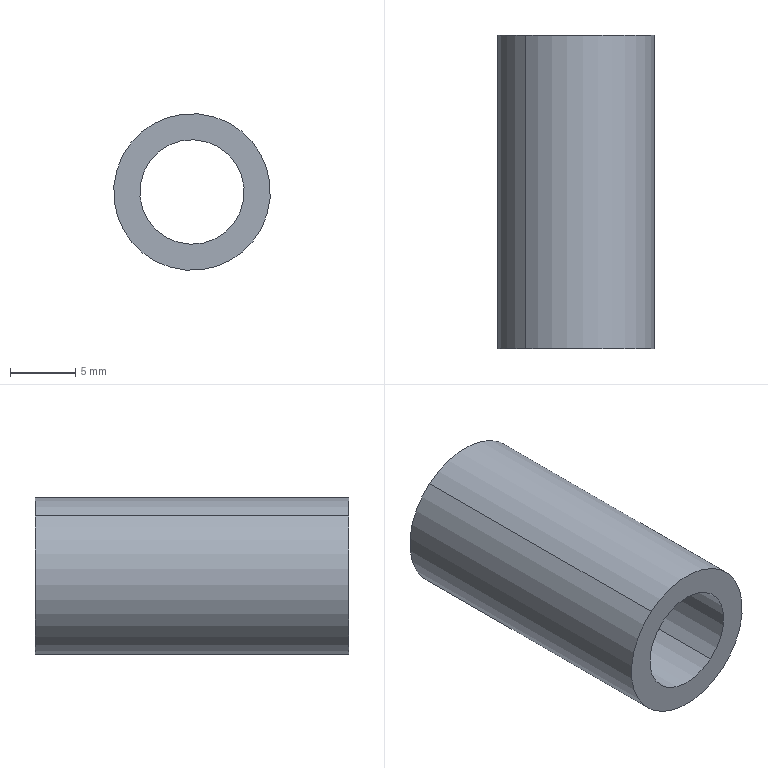Part | SolidWorks | features BaseBody 1 | 1 solid | 6 faces | box 12 x 24 x 12 mm | volume 1508 mm3 | cylinder 4 | plane 2 | commonest cylinder face diameters 8 x2 12 x2
STEP:
#1=CARTESIAN_POINT('',(374.241,-16.,154.364));
#2=VERTEX_POINT('',#1);
#3=CARTESIAN_POINT('',(379.383,-16.,148.236));
#4=VERTEX_POINT('',#3);
#5=CARTESIAN_POINT('',(376.812,-16.,151.3));
#6=DIRECTION('',(0.,1.,0.));
#7=DIRECTION('',(-0.6428,0.,0.766));
#8=AXIS2_PLACEMENT_3D('',#5,#6,#7);
#9=CIRCLE('',#8,4.);
#10=EDGE_CURVE('',#2,#4,#9,.T.);
#11=ORIENTED_EDGE('',*,*,#10,.F.);
#12=CARTESIAN_POINT('',(374.241,8.,154.364));
#13=VERTEX_POINT('',#12);
#14=CARTESIAN_POINT('',(374.241,-32.971,154.364));
#15=DIRECTION('',(0.,1.,0.));
#16=VECTOR('',#15,1000.);
#17=LINE('',#14,#16);
#18=EDGE_CURVE('',#2,#13,#17,.T.);
#19=ORIENTED_EDGE('',*,*,#18,.T.);
#20=CARTESIAN_POINT('',(379.383,8.,148.236));
#21=VERTEX_POINT('',#20);
#22=CARTESIAN_POINT('',(376.812,8.,151.3));
#23=DIRECTION('',(0.,-1.,0.));
#24=DIRECTION('',(0.6428,0.,-0.766));
#25=AXIS2_PLACEMENT_3D('',#22,#23,#24);
#26=CIRCLE('',#25,4.);
#27=EDGE_CURVE('',#21,#13,#26,.T.);
#28=ORIENTED_EDGE('',*,*,#27,.F.);
#29=CARTESIAN_POINT('',(379.383,-32.971,148.236));
#30=DIRECTION('',(0.,1.,0.));
#31=VECTOR('',#30,1000.);
#32=LINE('',#29,#31);
#33=EDGE_CURVE('',#4,#21,#32,.T.);
#34=ORIENTED_EDGE('',*,*,#33,.F.);
#35=EDGE_LOOP('',(#11,#19,#28,#34));
#36=FACE_OUTER_BOUND('',#35,.T.);
#37=CARTESIAN_POINT('',(376.812,-32.971,151.3));
#38=DIRECTION('',(0.,1.,0.));
#39=DIRECTION('',(0.6428,0.,-0.766));
#40=AXIS2_PLACEMENT_3D('',#37,#38,#39);
#41=CYLINDRICAL_SURFACE('',#40,4.);
#42=ADVANCED_FACE('',(#36),#41,.F.);
#43=CARTESIAN_POINT('',(372.956,-16.,155.896));
#44=VERTEX_POINT('',#43);
#45=CARTESIAN_POINT('',(380.669,-16.,146.704));
#46=VERTEX_POINT('',#45);
#47=CARTESIAN_POINT('',(376.812,-16.,151.3));
#48=DIRECTION('',(0.,-1.,0.));
#49=DIRECTION('',(-0.6428,0.,0.766));
#50=AXIS2_PLACEMENT_3D('',#47,#48,#49);
#51=CIRCLE('',#50,6.);
#52=EDGE_CURVE('',#44,#46,#51,.T.);
#53=ORIENTED_EDGE('',*,*,#52,.F.);
#54=CARTESIAN_POINT('',(372.956,8.,155.896));
#55=VERTEX_POINT('',#54);
#56=CARTESIAN_POINT('',(372.956,-32.971,155.896));
#57=DIRECTION('',(0.,1.,0.));
#58=VECTOR('',#57,1000.);
#59=LINE('',#56,#58);
#60=EDGE_CURVE('',#44,#55,#59,.T.);
#61=ORIENTED_EDGE('',*,*,#60,.T.);
#62=CARTESIAN_POINT('',(380.669,8.,146.704));
#63=VERTEX_POINT('',#62);
#64=CARTESIAN_POINT('',(376.812,8.,151.3));
#65=DIRECTION('',(0.,1.,0.));
#66=DIRECTION('',(-0.6428,0.,0.766));
#67=AXIS2_PLACEMENT_3D('',#64,#65,#66);
#68=CIRCLE('',#67,6.);
#69=EDGE_CURVE('',#63,#55,#68,.T.);
#70=ORIENTED_EDGE('',*,*,#69,.F.);
#71=CARTESIAN_POINT('',(380.669,-32.971,146.704));
#72=DIRECTION('',(0.,1.,0.));
#73=VECTOR('',#72,1000.);
#74=LINE('',#71,#73);
#75=EDGE_CURVE('',#46,#63,#74,.T.);
#76=ORIENTED_EDGE('',*,*,#75,.F.);
#77=EDGE_LOOP('',(#53,#61,#70,#76));
#78=FACE_OUTER_BOUND('',#77,.T.);
#79=CARTESIAN_POINT('',(376.812,-32.971,151.3));
#80=DIRECTION('',(0.,1.,0.));
#81=DIRECTION('',(0.6428,0.,-0.766));
#82=AXIS2_PLACEMENT_3D('',#79,#80,#81);
#83=CYLINDRICAL_SURFACE('',#82,6.);
#84=ADVANCED_FACE('',(#78),#83,.T.);
#85=ORIENTED_EDGE('',*,*,#27,.T.);
#86=CARTESIAN_POINT('',(376.812,8.,151.3));
#87=DIRECTION('',(0.,-1.,0.));
#88=DIRECTION('',(0.6428,0.,-0.766));
#89=AXIS2_PLACEMENT_3D('',#86,#87,#88);
#90=CIRCLE('',#89,4.);
#91=EDGE_CURVE('',#13,#21,#90,.T.);
#92=ORIENTED_EDGE('',*,*,#91,.T.);
#93=EDGE_LOOP('',(#85,#92));
#94=FACE_BOUND('',#93,.T.);
#95=ORIENTED_EDGE('',*,*,#69,.T.);
#96=CARTESIAN_POINT('',(376.812,8.,151.3));
#97=DIRECTION('',(0.,1.,0.));
#98=DIRECTION('',(-0.6428,0.,0.766));
#99=AXIS2_PLACEMENT_3D('',#96,#97,#98);
#100=CIRCLE('',#99,6.);
#101=EDGE_CURVE('',#55,#63,#100,.T.);
#102=ORIENTED_EDGE('',*,*,#101,.T.);
#103=EDGE_LOOP('',(#95,#102));
#104=FACE_OUTER_BOUND('',#103,.T.);
#105=CARTESIAN_POINT('',(376.812,8.,151.3));
#106=DIRECTION('',(0.,1.,0.));
#107=DIRECTION('',(1.,0.,0.));
#108=AXIS2_PLACEMENT_3D('',#105,#106,#107);
#109=PLANE('',#108);
#110=ADVANCED_FACE('',(#94,#104),#109,.T.);
#111=ORIENTED_EDGE('',*,*,#60,.F.);
#112=CARTESIAN_POINT('',(376.812,-16.,151.3));
#113=DIRECTION('',(0.,-1.,0.));
#114=DIRECTION('',(-0.6428,0.,0.766));
#115=AXIS2_PLACEMENT_3D('',#112,#113,#114);
#116=CIRCLE('',#115,6.);
#117=EDGE_CURVE('',#46,#44,#116,.T.);
#118=ORIENTED_EDGE('',*,*,#117,.F.);
#119=ORIENTED_EDGE('',*,*,#75,.T.);
#120=ORIENTED_EDGE('',*,*,#101,.F.);
#121=EDGE_LOOP('',(#111,#118,#119,#120));
#122=FACE_OUTER_BOUND('',#121,.T.);
#123=CARTESIAN_POINT('',(376.812,-32.971,151.3));
#124=DIRECTION('',(0.,1.,0.));
#125=DIRECTION('',(0.6428,0.,-0.766));
#126=AXIS2_PLACEMENT_3D('',#123,#124,#125);
#127=CYLINDRICAL_SURFACE('',#126,6.);
#128=ADVANCED_FACE('',(#122),#127,.T.);
#129=CARTESIAN_POINT('',(376.812,-16.,151.3));
#130=DIRECTION('',(0.,1.,0.));
#131=DIRECTION('',(-0.6428,0.,0.766));
#132=AXIS2_PLACEMENT_3D('',#129,#130,#131);
#133=CIRCLE('',#132,4.);
#134=EDGE_CURVE('',#4,#2,#133,.T.);
#135=ORIENTED_EDGE('',*,*,#134,.T.);
#136=ORIENTED_EDGE('',*,*,#10,.T.);
#137=EDGE_LOOP('',(#135,#136));
#138=FACE_BOUND('',#137,.T.);
#139=ORIENTED_EDGE('',*,*,#117,.T.);
#140=ORIENTED_EDGE('',*,*,#52,.T.);
#141=EDGE_LOOP('',(#139,#140));
#142=FACE_OUTER_BOUND('',#141,.T.);
#143=CARTESIAN_POINT('',(376.812,-16.,151.3));
#144=DIRECTION('',(0.,1.,0.));
#145=DIRECTION('',(1.,0.,0.));
#146=AXIS2_PLACEMENT_3D('',#143,#144,#145);
#147=PLANE('',#146);
#148=ADVANCED_FACE('',(#138,#142),#147,.F.);
#149=ORIENTED_EDGE('',*,*,#18,.F.);
#150=ORIENTED_EDGE('',*,*,#134,.F.);
#151=ORIENTED_EDGE('',*,*,#33,.T.);
#152=ORIENTED_EDGE('',*,*,#91,.F.);
#153=EDGE_LOOP('',(#149,#150,#151,#152));
#154=FACE_OUTER_BOUND('',#153,.T.);
#155=CARTESIAN_POINT('',(376.812,-32.971,151.3));
#156=DIRECTION('',(0.,1.,0.));
#157=DIRECTION('',(0.6428,0.,-0.766));
#158=AXIS2_PLACEMENT_3D('',#155,#156,#157);
#159=CYLINDRICAL_SURFACE('',#158,4.);
#160=ADVANCED_FACE('',(#154),#159,.F.);
#161=CLOSED_SHELL('',(#42,#84,#110,#128,#148,#160));
#162=MANIFOLD_SOLID_BREP('',#161);
#163=CARTESIAN_POINT('',(0.,0.,0.));
#164=DIRECTION('',(0.,0.,1.));
#165=DIRECTION('',(1.,0.,0.));
#166=AXIS2_PLACEMENT_3D('',#163,#164,#165);
#167=(LENGTH_UNIT()NAMED_UNIT(*)SI_UNIT(.MILLI.,.METRE.));
#168=UNCERTAINTY_MEASURE_WITH_UNIT(LENGTH_MEASURE(0.00001),#167,'','');
#169=(NAMED_UNIT(*)PLANE_ANGLE_UNIT()SI_UNIT($,.RADIAN.));
#170=(NAMED_UNIT(*)SI_UNIT($,.STERADIAN.)SOLID_ANGLE_UNIT());
#171=(GEOMETRIC_REPRESENTATION_CONTEXT(3)GLOBAL_UNCERTAINTY_ASSIGNED_CONTEXT((#168))GLOBAL_UNIT_ASSIGNED_CONTEXT((#167,#169,#170))REPRESENTATION_CONTEXT('',''));
#172=ADVANCED_BREP_SHAPE_REPRESENTATION('',(#162,#166),#171);